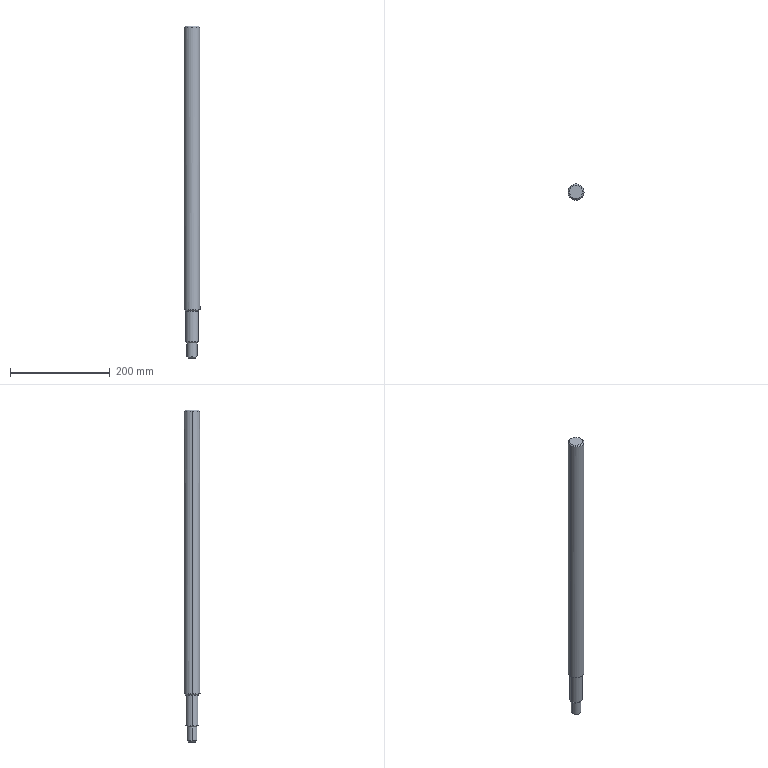Part | SolidWorks | features BaseBody 1 | 1 solid | 17 faces | box 32 x 32 x 664 mm | volume 498257 mm3 | cone 8 | cylinder 6 | plane 3 | commonest cylinder face diameters 20 x2 25 x2 32 x2
STEP:
#1=CARTESIAN_POINT('',(-16.,0.,661.5));
#2=VERTEX_POINT('',#1);
#3=CARTESIAN_POINT('',(16.,0.,661.5));
#4=VERTEX_POINT('',#3);
#5=CARTESIAN_POINT('',(0.,0.,661.5));
#6=DIRECTION('',(0.,0.,-1.));
#7=DIRECTION('',(-1.,0.,0.));
#8=AXIS2_PLACEMENT_3D('',#5,#6,#7);
#9=CIRCLE('',#8,16.);
#10=EDGE_CURVE('',#2,#4,#9,.T.);
#11=ORIENTED_EDGE('',*,*,#10,.T.);
#12=CARTESIAN_POINT('',(16.,0.,96.5));
#13=VERTEX_POINT('',#12);
#14=CARTESIAN_POINT('',(16.,0.,664.));
#15=DIRECTION('',(0.,0.,-1.));
#16=VECTOR('',#15,1000.);
#17=LINE('',#14,#16);
#18=EDGE_CURVE('',#4,#13,#17,.T.);
#19=ORIENTED_EDGE('',*,*,#18,.T.);
#20=CARTESIAN_POINT('',(0.,16.,96.5));
#21=VERTEX_POINT('',#20);
#22=CARTESIAN_POINT('',(0.,0.,96.5));
#23=DIRECTION('',(0.,0.,1.));
#24=DIRECTION('',(-1.,0.,0.));
#25=AXIS2_PLACEMENT_3D('',#22,#23,#24);
#26=CIRCLE('',#25,16.);
#27=EDGE_CURVE('',#13,#21,#26,.T.);
#28=ORIENTED_EDGE('',*,*,#27,.T.);
#29=CARTESIAN_POINT('',(-16.,0.,96.5));
#30=VERTEX_POINT('',#29);
#31=CARTESIAN_POINT('',(0.,0.,96.5));
#32=DIRECTION('',(0.,0.,1.));
#33=DIRECTION('',(-1.,0.,0.));
#34=AXIS2_PLACEMENT_3D('',#31,#32,#33);
#35=CIRCLE('',#34,16.);
#36=EDGE_CURVE('',#21,#30,#35,.T.);
#37=ORIENTED_EDGE('',*,*,#36,.T.);
#38=CARTESIAN_POINT('',(-16.,0.,664.));
#39=DIRECTION('',(0.,0.,-1.));
#40=VECTOR('',#39,1000.);
#41=LINE('',#38,#40);
#42=EDGE_CURVE('',#2,#30,#41,.T.);
#43=ORIENTED_EDGE('',*,*,#42,.F.);
#44=EDGE_LOOP('',(#11,#19,#28,#37,#43));
#45=FACE_OUTER_BOUND('',#44,.T.);
#46=CARTESIAN_POINT('',(0.,0.,664.));
#47=DIRECTION('',(0.,0.,-1.));
#48=DIRECTION('',(-1.,0.,0.));
#49=AXIS2_PLACEMENT_3D('',#46,#47,#48);
#50=CYLINDRICAL_SURFACE('',#49,16.);
#51=ADVANCED_FACE('',(#45),#50,.T.);
#52=CARTESIAN_POINT('',(0.,-13.5,94.));
#53=VERTEX_POINT('',#52);
#54=CARTESIAN_POINT('',(0.,13.5,94.));
#55=VERTEX_POINT('',#54);
#56=CARTESIAN_POINT('',(0.,0.,94.));
#57=DIRECTION('',(0.,0.,1.));
#58=DIRECTION('',(0.,-1.,0.));
#59=AXIS2_PLACEMENT_3D('',#56,#57,#58);
#60=CIRCLE('',#59,13.5);
#61=EDGE_CURVE('',#53,#55,#60,.T.);
#62=ORIENTED_EDGE('',*,*,#61,.T.);
#63=CARTESIAN_POINT('',(0.,16.,96.5));
#64=DIRECTION('',(0.,0.7071,0.7071));
#65=VECTOR('',#64,1000.);
#66=LINE('',#63,#65);
#67=EDGE_CURVE('',#55,#21,#66,.T.);
#68=ORIENTED_EDGE('',*,*,#67,.T.);
#69=ORIENTED_EDGE('',*,*,#27,.F.);
#70=CARTESIAN_POINT('',(0.,-16.,96.5));
#71=VERTEX_POINT('',#70);
#72=CARTESIAN_POINT('',(0.,0.,96.5));
#73=DIRECTION('',(0.,0.,1.));
#74=DIRECTION('',(-1.,0.,0.));
#75=AXIS2_PLACEMENT_3D('',#72,#73,#74);
#76=CIRCLE('',#75,16.);
#77=EDGE_CURVE('',#71,#13,#76,.T.);
#78=ORIENTED_EDGE('',*,*,#77,.F.);
#79=CARTESIAN_POINT('',(0.,-16.,96.5));
#80=DIRECTION('',(0.,-0.7071,0.7071));
#81=VECTOR('',#80,1000.);
#82=LINE('',#79,#81);
#83=EDGE_CURVE('',#53,#71,#82,.T.);
#84=ORIENTED_EDGE('',*,*,#83,.F.);
#85=EDGE_LOOP('',(#62,#68,#69,#78,#84));
#86=FACE_OUTER_BOUND('',#85,.T.);
#87=CARTESIAN_POINT('',(0.,0.,96.5));
#88=DIRECTION('',(0.,0.,1.));
#89=DIRECTION('',(0.,-1.,0.));
#90=AXIS2_PLACEMENT_3D('',#87,#88,#89);
#91=CONICAL_SURFACE('',#90,16.,0.7854);
#92=ADVANCED_FACE('',(#86),#91,.T.);
#93=CARTESIAN_POINT('',(-13.5,0.,664.));
#94=VERTEX_POINT('',#93);
#95=CARTESIAN_POINT('',(13.5,0.,664.));
#96=VERTEX_POINT('',#95);
#97=CARTESIAN_POINT('',(0.,0.,664.));
#98=DIRECTION('',(0.,0.,-1.));
#99=DIRECTION('',(-1.,0.,0.));
#100=AXIS2_PLACEMENT_3D('',#97,#98,#99);
#101=CIRCLE('',#100,13.5);
#102=EDGE_CURVE('',#94,#96,#101,.T.);
#103=ORIENTED_EDGE('',*,*,#102,.T.);
#104=CARTESIAN_POINT('',(16.,0.,661.5));
#105=DIRECTION('',(0.7071,0.,-0.7071));
#106=VECTOR('',#105,1000.);
#107=LINE('',#104,#106);
#108=EDGE_CURVE('',#96,#4,#107,.T.);
#109=ORIENTED_EDGE('',*,*,#108,.T.);
#110=ORIENTED_EDGE('',*,*,#10,.F.);
#111=CARTESIAN_POINT('',(-16.,0.,661.5));
#112=DIRECTION('',(-0.7071,0.,-0.7071));
#113=VECTOR('',#112,1000.);
#114=LINE('',#111,#113);
#115=EDGE_CURVE('',#94,#2,#114,.T.);
#116=ORIENTED_EDGE('',*,*,#115,.F.);
#117=EDGE_LOOP('',(#103,#109,#110,#116));
#118=FACE_OUTER_BOUND('',#117,.T.);
#119=CARTESIAN_POINT('',(0.,0.,661.5));
#120=DIRECTION('',(0.,0.,-1.));
#121=DIRECTION('',(-1.,0.,0.));
#122=AXIS2_PLACEMENT_3D('',#119,#120,#121);
#123=CONICAL_SURFACE('',#122,16.,0.7854);
#124=ADVANCED_FACE('',(#118),#123,.T.);
#125=CARTESIAN_POINT('',(-12.5,0.,94.));
#126=VERTEX_POINT('',#125);
#127=CARTESIAN_POINT('',(12.5,0.,94.));
#128=VERTEX_POINT('',#127);
#129=CARTESIAN_POINT('',(0.,0.,94.));
#130=DIRECTION('',(0.,0.,-1.));
#131=DIRECTION('',(-1.,0.,0.));
#132=AXIS2_PLACEMENT_3D('',#129,#130,#131);
#133=CIRCLE('',#132,12.5);
#134=EDGE_CURVE('',#126,#128,#133,.T.);
#135=ORIENTED_EDGE('',*,*,#134,.T.);
#136=CARTESIAN_POINT('',(12.5,0.,32.5));
#137=VERTEX_POINT('',#136);
#138=CARTESIAN_POINT('',(12.5,0.,94.));
#139=DIRECTION('',(0.,0.,-1.));
#140=VECTOR('',#139,1000.);
#141=LINE('',#138,#140);
#142=EDGE_CURVE('',#128,#137,#141,.T.);
#143=ORIENTED_EDGE('',*,*,#142,.T.);
#144=CARTESIAN_POINT('',(-12.5,0.,32.5));
#145=VERTEX_POINT('',#144);
#146=CARTESIAN_POINT('',(0.,0.,32.5));
#147=DIRECTION('',(0.,0.,1.));
#148=DIRECTION('',(-1.,0.,0.));
#149=AXIS2_PLACEMENT_3D('',#146,#147,#148);
#150=CIRCLE('',#149,12.5);
#151=EDGE_CURVE('',#137,#145,#150,.T.);
#152=ORIENTED_EDGE('',*,*,#151,.T.);
#153=CARTESIAN_POINT('',(-12.5,0.,94.));
#154=DIRECTION('',(0.,0.,-1.));
#155=VECTOR('',#154,1000.);
#156=LINE('',#153,#155);
#157=EDGE_CURVE('',#126,#145,#156,.T.);
#158=ORIENTED_EDGE('',*,*,#157,.F.);
#159=EDGE_LOOP('',(#135,#143,#152,#158));
#160=FACE_OUTER_BOUND('',#159,.T.);
#161=CARTESIAN_POINT('',(0.,0.,94.));
#162=DIRECTION('',(0.,0.,-1.));
#163=DIRECTION('',(-1.,0.,0.));
#164=AXIS2_PLACEMENT_3D('',#161,#162,#163);
#165=CYLINDRICAL_SURFACE('',#164,12.5);
#166=ADVANCED_FACE('',(#160),#165,.T.);
#167=CARTESIAN_POINT('',(10.,0.,30.));
#168=VERTEX_POINT('',#167);
#169=CARTESIAN_POINT('',(-10.,0.,30.));
#170=VERTEX_POINT('',#169);
#171=CARTESIAN_POINT('',(0.,0.,30.));
#172=DIRECTION('',(0.,0.,1.));
#173=DIRECTION('',(-1.,0.,0.));
#174=AXIS2_PLACEMENT_3D('',#171,#172,#173);
#175=CIRCLE('',#174,10.);
#176=EDGE_CURVE('',#168,#170,#175,.T.);
#177=ORIENTED_EDGE('',*,*,#176,.T.);
#178=CARTESIAN_POINT('',(-12.5,0.,32.5));
#179=DIRECTION('',(-0.7071,0.,0.7071));
#180=VECTOR('',#179,1000.);
#181=LINE('',#178,#180);
#182=EDGE_CURVE('',#170,#145,#181,.T.);
#183=ORIENTED_EDGE('',*,*,#182,.T.);
#184=ORIENTED_EDGE('',*,*,#151,.F.);
#185=CARTESIAN_POINT('',(12.5,0.,32.5));
#186=DIRECTION('',(0.7071,0.,0.7071));
#187=VECTOR('',#186,1000.);
#188=LINE('',#185,#187);
#189=EDGE_CURVE('',#168,#137,#188,.T.);
#190=ORIENTED_EDGE('',*,*,#189,.F.);
#191=EDGE_LOOP('',(#177,#183,#184,#190));
#192=FACE_OUTER_BOUND('',#191,.T.);
#193=CARTESIAN_POINT('',(0.,0.,32.5));
#194=DIRECTION('',(0.,0.,1.));
#195=DIRECTION('',(1.,0.,0.));
#196=AXIS2_PLACEMENT_3D('',#193,#194,#195);
#197=CONICAL_SURFACE('',#196,12.5,0.7854);
#198=ADVANCED_FACE('',(#192),#197,.T.);
#199=ORIENTED_EDGE('',*,*,#176,.F.);
#200=CARTESIAN_POINT('',(10.,0.,2.5));
#201=VERTEX_POINT('',#200);
#202=CARTESIAN_POINT('',(10.,0.,30.));
#203=DIRECTION('',(0.,0.,-1.));
#204=VECTOR('',#203,1000.);
#205=LINE('',#202,#204);
#206=EDGE_CURVE('',#168,#201,#205,.T.);
#207=ORIENTED_EDGE('',*,*,#206,.T.);
#208=CARTESIAN_POINT('',(-10.,0.,2.5));
#209=VERTEX_POINT('',#208);
#210=CARTESIAN_POINT('',(0.,0.,2.5));
#211=DIRECTION('',(0.,0.,1.));
#212=DIRECTION('',(-1.,0.,0.));
#213=AXIS2_PLACEMENT_3D('',#210,#211,#212);
#214=CIRCLE('',#213,10.);
#215=EDGE_CURVE('',#201,#209,#214,.T.);
#216=ORIENTED_EDGE('',*,*,#215,.T.);
#217=CARTESIAN_POINT('',(-10.,0.,30.));
#218=DIRECTION('',(0.,0.,-1.));
#219=VECTOR('',#218,1000.);
#220=LINE('',#217,#219);
#221=EDGE_CURVE('',#170,#209,#220,.T.);
#222=ORIENTED_EDGE('',*,*,#221,.F.);
#223=EDGE_LOOP('',(#199,#207,#216,#222));
#224=FACE_OUTER_BOUND('',#223,.T.);
#225=CARTESIAN_POINT('',(0.,0.,30.));
#226=DIRECTION('',(0.,0.,-1.));
#227=DIRECTION('',(-1.,0.,0.));
#228=AXIS2_PLACEMENT_3D('',#225,#226,#227);
#229=CYLINDRICAL_SURFACE('',#228,10.);
#230=ADVANCED_FACE('',(#224),#229,.T.);
#231=CARTESIAN_POINT('',(7.5,0.,0.));
#232=VERTEX_POINT('',#231);
#233=CARTESIAN_POINT('',(-7.5,0.,0.));
#234=VERTEX_POINT('',#233);
#235=CARTESIAN_POINT('',(0.,0.,0.));
#236=DIRECTION('',(0.,0.,1.));
#237=DIRECTION('',(1.,0.,0.));
#238=AXIS2_PLACEMENT_3D('',#235,#236,#237);
#239=CIRCLE('',#238,7.5);
#240=EDGE_CURVE('',#232,#234,#239,.T.);
#241=ORIENTED_EDGE('',*,*,#240,.T.);
#242=CARTESIAN_POINT('',(-10.,0.,2.5));
#243=DIRECTION('',(-0.7071,0.,0.7071));
#244=VECTOR('',#243,1000.);
#245=LINE('',#242,#244);
#246=EDGE_CURVE('',#234,#209,#245,.T.);
#247=ORIENTED_EDGE('',*,*,#246,.T.);
#248=ORIENTED_EDGE('',*,*,#215,.F.);
#249=CARTESIAN_POINT('',(10.,0.,2.5));
#250=DIRECTION('',(0.7071,0.,0.7071));
#251=VECTOR('',#250,1000.);
#252=LINE('',#249,#251);
#253=EDGE_CURVE('',#232,#201,#252,.T.);
#254=ORIENTED_EDGE('',*,*,#253,.F.);
#255=EDGE_LOOP('',(#241,#247,#248,#254));
#256=FACE_OUTER_BOUND('',#255,.T.);
#257=CARTESIAN_POINT('',(0.,0.,2.5));
#258=DIRECTION('',(0.,0.,1.));
#259=DIRECTION('',(1.,0.,0.));
#260=AXIS2_PLACEMENT_3D('',#257,#258,#259);
#261=CONICAL_SURFACE('',#260,10.,0.7854);
#262=ADVANCED_FACE('',(#256),#261,.T.);
#263=ORIENTED_EDGE('',*,*,#18,.F.);
#264=CARTESIAN_POINT('',(0.,0.,661.5));
#265=DIRECTION('',(0.,0.,-1.));
#266=DIRECTION('',(-1.,0.,0.));
#267=AXIS2_PLACEMENT_3D('',#264,#265,#266);
#268=CIRCLE('',#267,16.);
#269=EDGE_CURVE('',#4,#2,#268,.T.);
#270=ORIENTED_EDGE('',*,*,#269,.T.);
#271=ORIENTED_EDGE('',*,*,#42,.T.);
#272=CARTESIAN_POINT('',(0.,0.,96.5));
#273=DIRECTION('',(0.,0.,1.));
#274=DIRECTION('',(-1.,0.,0.));
#275=AXIS2_PLACEMENT_3D('',#272,#273,#274);
#276=CIRCLE('',#275,16.);
#277=EDGE_CURVE('',#30,#71,#276,.T.);
#278=ORIENTED_EDGE('',*,*,#277,.T.);
#279=ORIENTED_EDGE('',*,*,#77,.T.);
#280=EDGE_LOOP('',(#263,#270,#271,#278,#279));
#281=FACE_OUTER_BOUND('',#280,.T.);
#282=CARTESIAN_POINT('',(0.,0.,664.));
#283=DIRECTION('',(0.,0.,-1.));
#284=DIRECTION('',(-1.,0.,0.));
#285=AXIS2_PLACEMENT_3D('',#282,#283,#284);
#286=CYLINDRICAL_SURFACE('',#285,16.);
#287=ADVANCED_FACE('',(#281),#286,.T.);
#288=ORIENTED_EDGE('',*,*,#67,.F.);
#289=CARTESIAN_POINT('',(0.,0.,94.));
#290=DIRECTION('',(0.,0.,1.));
#291=DIRECTION('',(0.,-1.,0.));
#292=AXIS2_PLACEMENT_3D('',#289,#290,#291);
#293=CIRCLE('',#292,13.5);
#294=EDGE_CURVE('',#55,#53,#293,.T.);
#295=ORIENTED_EDGE('',*,*,#294,.T.);
#296=ORIENTED_EDGE('',*,*,#83,.T.);
#297=ORIENTED_EDGE('',*,*,#277,.F.);
#298=ORIENTED_EDGE('',*,*,#36,.F.);
#299=EDGE_LOOP('',(#288,#295,#296,#297,#298));
#300=FACE_OUTER_BOUND('',#299,.T.);
#301=CARTESIAN_POINT('',(0.,0.,96.5));
#302=DIRECTION('',(0.,0.,1.));
#303=DIRECTION('',(0.,-1.,0.));
#304=AXIS2_PLACEMENT_3D('',#301,#302,#303);
#305=CONICAL_SURFACE('',#304,16.,0.7854);
#306=ADVANCED_FACE('',(#300),#305,.T.);
#307=ORIENTED_EDGE('',*,*,#108,.F.);
#308=CARTESIAN_POINT('',(0.,0.,664.));
#309=DIRECTION('',(0.,0.,-1.));
#310=DIRECTION('',(-1.,0.,0.));
#311=AXIS2_PLACEMENT_3D('',#308,#309,#310);
#312=CIRCLE('',#311,13.5);
#313=EDGE_CURVE('',#96,#94,#312,.T.);
#314=ORIENTED_EDGE('',*,*,#313,.T.);
#315=ORIENTED_EDGE('',*,*,#115,.T.);
#316=ORIENTED_EDGE('',*,*,#269,.F.);
#317=EDGE_LOOP('',(#307,#314,#315,#316));
#318=FACE_OUTER_BOUND('',#317,.T.);
#319=CARTESIAN_POINT('',(0.,0.,661.5));
#320=DIRECTION('',(0.,0.,-1.));
#321=DIRECTION('',(-1.,0.,0.));
#322=AXIS2_PLACEMENT_3D('',#319,#320,#321);
#323=CONICAL_SURFACE('',#322,16.,0.7854);
#324=ADVANCED_FACE('',(#318),#323,.T.);
#325=ORIENTED_EDGE('',*,*,#134,.F.);
#326=CARTESIAN_POINT('',(0.,0.,94.));
#327=DIRECTION('',(0.,0.,-1.));
#328=DIRECTION('',(-1.,0.,0.));
#329=AXIS2_PLACEMENT_3D('',#326,#327,#328);
#330=CIRCLE('',#329,12.5);
#331=EDGE_CURVE('',#128,#126,#330,.T.);
#332=ORIENTED_EDGE('',*,*,#331,.F.);
#333=EDGE_LOOP('',(#325,#332));
#334=FACE_BOUND('',#333,.T.);
#335=ORIENTED_EDGE('',*,*,#61,.F.);
#336=ORIENTED_EDGE('',*,*,#294,.F.);
#337=EDGE_LOOP('',(#335,#336));
#338=FACE_OUTER_BOUND('',#337,.T.);
#339=CARTESIAN_POINT('',(0.,0.,94.));
#340=DIRECTION('',(0.,0.,1.));
#341=DIRECTION('',(1.,0.,0.));
#342=AXIS2_PLACEMENT_3D('',#339,#340,#341);
#343=PLANE('',#342);
#344=ADVANCED_FACE('',(#334,#338),#343,.F.);
#345=ORIENTED_EDGE('',*,*,#102,.F.);
#346=ORIENTED_EDGE('',*,*,#313,.F.);
#347=EDGE_LOOP('',(#345,#346));
#348=FACE_OUTER_BOUND('',#347,.T.);
#349=CARTESIAN_POINT('',(0.,0.,664.));
#350=DIRECTION('',(0.,0.,1.));
#351=DIRECTION('',(1.,0.,0.));
#352=AXIS2_PLACEMENT_3D('',#349,#350,#351);
#353=PLANE('',#352);
#354=ADVANCED_FACE('',(#348),#353,.T.);
#355=ORIENTED_EDGE('',*,*,#142,.F.);
#356=ORIENTED_EDGE('',*,*,#331,.T.);
#357=ORIENTED_EDGE('',*,*,#157,.T.);
#358=CARTESIAN_POINT('',(0.,0.,32.5));
#359=DIRECTION('',(0.,0.,1.));
#360=DIRECTION('',(-1.,0.,0.));
#361=AXIS2_PLACEMENT_3D('',#358,#359,#360);
#362=CIRCLE('',#361,12.5);
#363=EDGE_CURVE('',#145,#137,#362,.T.);
#364=ORIENTED_EDGE('',*,*,#363,.T.);
#365=EDGE_LOOP('',(#355,#356,#357,#364));
#366=FACE_OUTER_BOUND('',#365,.T.);
#367=CARTESIAN_POINT('',(0.,0.,94.));
#368=DIRECTION('',(0.,0.,-1.));
#369=DIRECTION('',(-1.,0.,0.));
#370=AXIS2_PLACEMENT_3D('',#367,#368,#369);
#371=CYLINDRICAL_SURFACE('',#370,12.5);
#372=ADVANCED_FACE('',(#366),#371,.T.);
#373=ORIENTED_EDGE('',*,*,#182,.F.);
#374=CARTESIAN_POINT('',(0.,0.,30.));
#375=DIRECTION('',(0.,0.,1.));
#376=DIRECTION('',(-1.,0.,0.));
#377=AXIS2_PLACEMENT_3D('',#374,#375,#376);
#378=CIRCLE('',#377,10.);
#379=EDGE_CURVE('',#170,#168,#378,.T.);
#380=ORIENTED_EDGE('',*,*,#379,.T.);
#381=ORIENTED_EDGE('',*,*,#189,.T.);
#382=ORIENTED_EDGE('',*,*,#363,.F.);
#383=EDGE_LOOP('',(#373,#380,#381,#382));
#384=FACE_OUTER_BOUND('',#383,.T.);
#385=CARTESIAN_POINT('',(0.,0.,32.5));
#386=DIRECTION('',(0.,0.,1.));
#387=DIRECTION('',(1.,0.,0.));
#388=AXIS2_PLACEMENT_3D('',#385,#386,#387);
#389=CONICAL_SURFACE('',#388,12.5,0.7854);
#390=ADVANCED_FACE('',(#384),#389,.T.);
#391=ORIENTED_EDGE('',*,*,#206,.F.);
#392=ORIENTED_EDGE('',*,*,#379,.F.);
#393=ORIENTED_EDGE('',*,*,#221,.T.);
#394=CARTESIAN_POINT('',(0.,0.,2.5));
#395=DIRECTION('',(0.,0.,1.));
#396=DIRECTION('',(-1.,0.,0.));
#397=AXIS2_PLACEMENT_3D('',#394,#395,#396);
#398=CIRCLE('',#397,10.);
#399=EDGE_CURVE('',#209,#201,#398,.T.);
#400=ORIENTED_EDGE('',*,*,#399,.T.);
#401=EDGE_LOOP('',(#391,#392,#393,#400));
#402=FACE_OUTER_BOUND('',#401,.T.);
#403=CARTESIAN_POINT('',(0.,0.,30.));
#404=DIRECTION('',(0.,0.,-1.));
#405=DIRECTION('',(-1.,0.,0.));
#406=AXIS2_PLACEMENT_3D('',#403,#404,#405);
#407=CYLINDRICAL_SURFACE('',#406,10.);
#408=ADVANCED_FACE('',(#402),#407,.T.);
#409=ORIENTED_EDGE('',*,*,#246,.F.);
#410=CARTESIAN_POINT('',(0.,0.,0.));
#411=DIRECTION('',(0.,0.,1.));
#412=DIRECTION('',(1.,0.,0.));
#413=AXIS2_PLACEMENT_3D('',#410,#411,#412);
#414=CIRCLE('',#413,7.5);
#415=EDGE_CURVE('',#234,#232,#414,.T.);
#416=ORIENTED_EDGE('',*,*,#415,.T.);
#417=ORIENTED_EDGE('',*,*,#253,.T.);
#418=ORIENTED_EDGE('',*,*,#399,.F.);
#419=EDGE_LOOP('',(#409,#416,#417,#418));
#420=FACE_OUTER_BOUND('',#419,.T.);
#421=CARTESIAN_POINT('',(0.,0.,2.5));
#422=DIRECTION('',(0.,0.,1.));
#423=DIRECTION('',(1.,0.,0.));
#424=AXIS2_PLACEMENT_3D('',#421,#422,#423);
#425=CONICAL_SURFACE('',#424,10.,0.7854);
#426=ADVANCED_FACE('',(#420),#425,.T.);
#427=ORIENTED_EDGE('',*,*,#240,.F.);
#428=ORIENTED_EDGE('',*,*,#415,.F.);
#429=EDGE_LOOP('',(#427,#428));
#430=FACE_OUTER_BOUND('',#429,.T.);
#431=CARTESIAN_POINT('',(0.,0.,0.));
#432=DIRECTION('',(0.,0.,1.));
#433=DIRECTION('',(1.,0.,0.));
#434=AXIS2_PLACEMENT_3D('',#431,#432,#433);
#435=PLANE('',#434);
#436=ADVANCED_FACE('',(#430),#435,.F.);
#437=CLOSED_SHELL('',(#51,#92,#124,#166,#198,#230,#262,#287,#306,#324,#344,#354,#372,#390,#408,#426,#436));
#438=MANIFOLD_SOLID_BREP('',#437);
#439=CARTESIAN_POINT('',(0.,0.,0.));
#440=DIRECTION('',(0.,0.,1.));
#441=DIRECTION('',(1.,0.,0.));
#442=AXIS2_PLACEMENT_3D('',#439,#440,#441);
#443=(LENGTH_UNIT()NAMED_UNIT(*)SI_UNIT(.MILLI.,.METRE.));
#444=UNCERTAINTY_MEASURE_WITH_UNIT(LENGTH_MEASURE(0.00001),#443,'','');
#445=(NAMED_UNIT(*)PLANE_ANGLE_UNIT()SI_UNIT($,.RADIAN.));
#446=(NAMED_UNIT(*)SI_UNIT($,.STERADIAN.)SOLID_ANGLE_UNIT());
#447=(GEOMETRIC_REPRESENTATION_CONTEXT(3)GLOBAL_UNCERTAINTY_ASSIGNED_CONTEXT((#444))GLOBAL_UNIT_ASSIGNED_CONTEXT((#443,#445,#446))REPRESENTATION_CONTEXT('',''));
#448=ADVANCED_BREP_SHAPE_REPRESENTATION('',(#438,#442),#447);